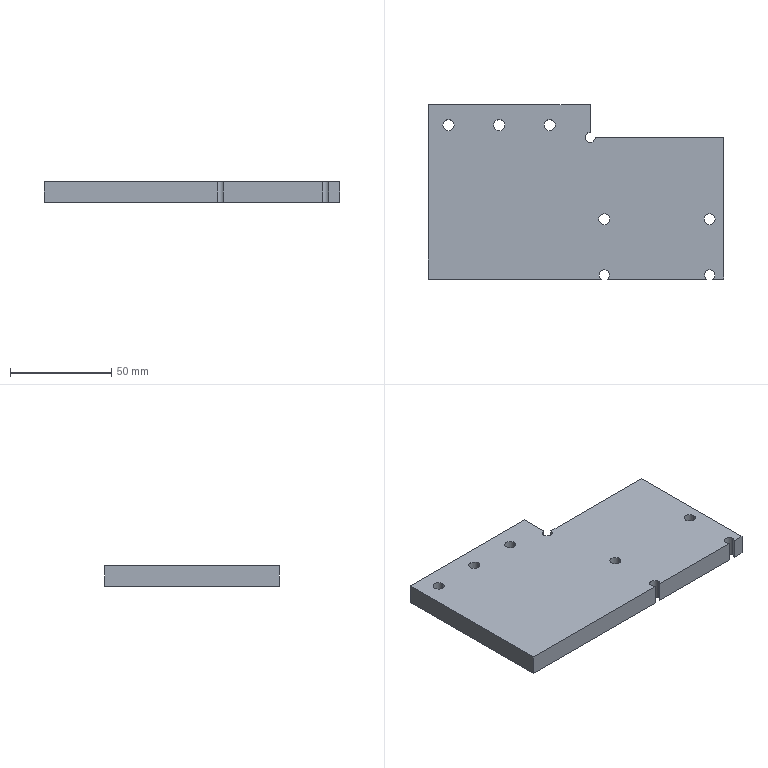Part | STEP file | 10-22Z轴连接块B | 1 solid | 43 faces | box 146 x 86 x 10 mm | volume 111813 mm3 | cylinder 28 | plane 15 | commonest cylinder face diameters 5.5 x10 10 x10 5 x8
STEP:
#1=CARTESIAN_POINT('',(16.5,-41.,10.));
#2=VERTEX_POINT('',#1);
#3=CARTESIAN_POINT('',(15.5,-43.,10.));
#4=VERTEX_POINT('',#3);
#5=CARTESIAN_POINT('',(14.,-41.,10.));
#6=DIRECTION('',(0.,0.,-1.));
#7=DIRECTION('',(-1.,0.,0.));
#8=AXIS2_PLACEMENT_3D('',#5,#6,#7);
#9=CIRCLE('',#8,2.5);
#10=EDGE_CURVE('',#2,#4,#9,.T.);
#11=ORIENTED_EDGE('',*,*,#10,.F.);
#12=CARTESIAN_POINT('',(16.5,-41.,0.));
#13=VERTEX_POINT('',#12);
#14=CARTESIAN_POINT('',(16.5,-41.,10.));
#15=DIRECTION('',(0.,0.,-1.));
#16=VECTOR('',#15,1000.);
#17=LINE('',#14,#16);
#18=EDGE_CURVE('',#2,#13,#17,.T.);
#19=ORIENTED_EDGE('',*,*,#18,.T.);
#20=CARTESIAN_POINT('',(15.5,-43.,0.));
#21=VERTEX_POINT('',#20);
#22=CARTESIAN_POINT('',(14.,-41.,0.));
#23=DIRECTION('',(0.,0.,1.));
#24=DIRECTION('',(1.,0.,0.));
#25=AXIS2_PLACEMENT_3D('',#22,#23,#24);
#26=CIRCLE('',#25,2.5);
#27=EDGE_CURVE('',#21,#13,#26,.T.);
#28=ORIENTED_EDGE('',*,*,#27,.F.);
#29=CARTESIAN_POINT('',(15.5,-43.,10.));
#30=DIRECTION('',(0.,0.,-1.));
#31=VECTOR('',#30,1000.);
#32=LINE('',#29,#31);
#33=EDGE_CURVE('',#4,#21,#32,.T.);
#34=ORIENTED_EDGE('',*,*,#33,.F.);
#35=EDGE_LOOP('',(#11,#19,#28,#34));
#36=FACE_OUTER_BOUND('',#35,.T.);
#37=CARTESIAN_POINT('',(14.,-41.,10.));
#38=DIRECTION('',(0.,0.,-1.));
#39=DIRECTION('',(-1.,0.,0.));
#40=AXIS2_PLACEMENT_3D('',#37,#38,#39);
#41=CYLINDRICAL_SURFACE('',#40,2.5);
#42=ADVANCED_FACE('',(#36),#41,.F.);
#43=ORIENTED_EDGE('',*,*,#18,.F.);
#44=CARTESIAN_POINT('',(11.5,-41.,10.));
#45=VERTEX_POINT('',#44);
#46=CARTESIAN_POINT('',(14.,-41.,10.));
#47=DIRECTION('',(0.,0.,-1.));
#48=DIRECTION('',(-1.,0.,0.));
#49=AXIS2_PLACEMENT_3D('',#46,#47,#48);
#50=CIRCLE('',#49,2.5);
#51=EDGE_CURVE('',#45,#2,#50,.T.);
#52=ORIENTED_EDGE('',*,*,#51,.F.);
#53=CARTESIAN_POINT('',(11.5,-41.,0.));
#54=VERTEX_POINT('',#53);
#55=CARTESIAN_POINT('',(11.5,-41.,10.));
#56=DIRECTION('',(0.,0.,-1.));
#57=VECTOR('',#56,1000.);
#58=LINE('',#55,#57);
#59=EDGE_CURVE('',#45,#54,#58,.T.);
#60=ORIENTED_EDGE('',*,*,#59,.T.);
#61=CARTESIAN_POINT('',(14.,-41.,0.));
#62=DIRECTION('',(0.,0.,1.));
#63=DIRECTION('',(1.,0.,0.));
#64=AXIS2_PLACEMENT_3D('',#61,#62,#63);
#65=CIRCLE('',#64,2.5);
#66=EDGE_CURVE('',#13,#54,#65,.T.);
#67=ORIENTED_EDGE('',*,*,#66,.F.);
#68=EDGE_LOOP('',(#43,#52,#60,#67));
#69=FACE_OUTER_BOUND('',#68,.T.);
#70=CARTESIAN_POINT('',(14.,-41.,10.));
#71=DIRECTION('',(0.,0.,-1.));
#72=DIRECTION('',(-1.,0.,0.));
#73=AXIS2_PLACEMENT_3D('',#70,#71,#72);
#74=CYLINDRICAL_SURFACE('',#73,2.5);
#75=ADVANCED_FACE('',(#69),#74,.F.);
#76=CARTESIAN_POINT('',(68.5,-41.,10.));
#77=VERTEX_POINT('',#76);
#78=CARTESIAN_POINT('',(67.5,-43.,10.));
#79=VERTEX_POINT('',#78);
#80=CARTESIAN_POINT('',(66.,-41.,10.));
#81=DIRECTION('',(0.,0.,-1.));
#82=DIRECTION('',(-1.,0.,0.));
#83=AXIS2_PLACEMENT_3D('',#80,#81,#82);
#84=CIRCLE('',#83,2.5);
#85=EDGE_CURVE('',#77,#79,#84,.T.);
#86=ORIENTED_EDGE('',*,*,#85,.F.);
#87=CARTESIAN_POINT('',(68.5,-41.,0.));
#88=VERTEX_POINT('',#87);
#89=CARTESIAN_POINT('',(68.5,-41.,10.));
#90=DIRECTION('',(0.,0.,-1.));
#91=VECTOR('',#90,1000.);
#92=LINE('',#89,#91);
#93=EDGE_CURVE('',#77,#88,#92,.T.);
#94=ORIENTED_EDGE('',*,*,#93,.T.);
#95=CARTESIAN_POINT('',(67.5,-43.,0.));
#96=VERTEX_POINT('',#95);
#97=CARTESIAN_POINT('',(66.,-41.,0.));
#98=DIRECTION('',(0.,0.,1.));
#99=DIRECTION('',(1.,0.,0.));
#100=AXIS2_PLACEMENT_3D('',#97,#98,#99);
#101=CIRCLE('',#100,2.5);
#102=EDGE_CURVE('',#96,#88,#101,.T.);
#103=ORIENTED_EDGE('',*,*,#102,.F.);
#104=CARTESIAN_POINT('',(67.5,-43.,10.));
#105=DIRECTION('',(0.,0.,-1.));
#106=VECTOR('',#105,1000.);
#107=LINE('',#104,#106);
#108=EDGE_CURVE('',#79,#96,#107,.T.);
#109=ORIENTED_EDGE('',*,*,#108,.F.);
#110=EDGE_LOOP('',(#86,#94,#103,#109));
#111=FACE_OUTER_BOUND('',#110,.T.);
#112=CARTESIAN_POINT('',(66.,-41.,10.));
#113=DIRECTION('',(0.,0.,-1.));
#114=DIRECTION('',(-1.,0.,0.));
#115=AXIS2_PLACEMENT_3D('',#112,#113,#114);
#116=CYLINDRICAL_SURFACE('',#115,2.5);
#117=ADVANCED_FACE('',(#111),#116,.F.);
#118=ORIENTED_EDGE('',*,*,#93,.F.);
#119=CARTESIAN_POINT('',(63.5,-41.,10.));
#120=VERTEX_POINT('',#119);
#121=CARTESIAN_POINT('',(66.,-41.,10.));
#122=DIRECTION('',(0.,0.,-1.));
#123=DIRECTION('',(-1.,0.,0.));
#124=AXIS2_PLACEMENT_3D('',#121,#122,#123);
#125=CIRCLE('',#124,2.5);
#126=EDGE_CURVE('',#120,#77,#125,.T.);
#127=ORIENTED_EDGE('',*,*,#126,.F.);
#128=CARTESIAN_POINT('',(63.5,-41.,0.));
#129=VERTEX_POINT('',#128);
#130=CARTESIAN_POINT('',(63.5,-41.,10.));
#131=DIRECTION('',(0.,0.,-1.));
#132=VECTOR('',#131,1000.);
#133=LINE('',#130,#132);
#134=EDGE_CURVE('',#120,#129,#133,.T.);
#135=ORIENTED_EDGE('',*,*,#134,.T.);
#136=CARTESIAN_POINT('',(66.,-41.,0.));
#137=DIRECTION('',(0.,0.,1.));
#138=DIRECTION('',(1.,0.,0.));
#139=AXIS2_PLACEMENT_3D('',#136,#137,#138);
#140=CIRCLE('',#139,2.5);
#141=EDGE_CURVE('',#88,#129,#140,.T.);
#142=ORIENTED_EDGE('',*,*,#141,.F.);
#143=EDGE_LOOP('',(#118,#127,#135,#142));
#144=FACE_OUTER_BOUND('',#143,.T.);
#145=CARTESIAN_POINT('',(66.,-41.,10.));
#146=DIRECTION('',(0.,0.,-1.));
#147=DIRECTION('',(-1.,0.,0.));
#148=AXIS2_PLACEMENT_3D('',#145,#146,#147);
#149=CYLINDRICAL_SURFACE('',#148,2.5);
#150=ADVANCED_FACE('',(#144),#149,.F.);
#151=CARTESIAN_POINT('',(71.,-13.5,5.4));
#152=VERTEX_POINT('',#151);
#153=CARTESIAN_POINT('',(61.,-13.5,5.4));
#154=VERTEX_POINT('',#153);
#155=CARTESIAN_POINT('',(66.,-13.5,5.4));
#156=DIRECTION('',(0.,0.,-1.));
#157=DIRECTION('',(-1.,0.,0.));
#158=AXIS2_PLACEMENT_3D('',#155,#156,#157);
#159=CIRCLE('',#158,5.);
#160=EDGE_CURVE('',#152,#154,#159,.T.);
#161=ORIENTED_EDGE('',*,*,#160,.F.);
#162=CARTESIAN_POINT('',(71.,-13.5,0.));
#163=VERTEX_POINT('',#162);
#164=CARTESIAN_POINT('',(71.,-13.5,0.));
#165=DIRECTION('',(0.,0.,-1.));
#166=VECTOR('',#165,1000.);
#167=LINE('',#164,#166);
#168=EDGE_CURVE('',#152,#163,#167,.T.);
#169=ORIENTED_EDGE('',*,*,#168,.T.);
#170=CARTESIAN_POINT('',(61.,-13.5,0.));
#171=VERTEX_POINT('',#170);
#172=CARTESIAN_POINT('',(66.,-13.5,0.));
#173=DIRECTION('',(0.,0.,-1.));
#174=DIRECTION('',(-1.,0.,0.));
#175=AXIS2_PLACEMENT_3D('',#172,#173,#174);
#176=CIRCLE('',#175,5.);
#177=EDGE_CURVE('',#163,#171,#176,.T.);
#178=ORIENTED_EDGE('',*,*,#177,.T.);
#179=CARTESIAN_POINT('',(61.,-13.5,0.));
#180=DIRECTION('',(0.,0.,-1.));
#181=VECTOR('',#180,1000.);
#182=LINE('',#179,#181);
#183=EDGE_CURVE('',#154,#171,#182,.T.);
#184=ORIENTED_EDGE('',*,*,#183,.F.);
#185=EDGE_LOOP('',(#161,#169,#178,#184));
#186=FACE_OUTER_BOUND('',#185,.T.);
#187=CARTESIAN_POINT('',(66.,-13.5,0.));
#188=DIRECTION('',(0.,0.,-1.));
#189=DIRECTION('',(-1.,0.,0.));
#190=AXIS2_PLACEMENT_3D('',#187,#188,#189);
#191=CYLINDRICAL_SURFACE('',#190,5.);
#192=ADVANCED_FACE('',(#186),#191,.F.);
#193=CARTESIAN_POINT('',(68.75,-13.5,10.));
#194=VERTEX_POINT('',#193);
#195=CARTESIAN_POINT('',(63.25,-13.5,10.));
#196=VERTEX_POINT('',#195);
#197=CARTESIAN_POINT('',(66.,-13.5,10.));
#198=DIRECTION('',(0.,0.,-1.));
#199=DIRECTION('',(-1.,0.,0.));
#200=AXIS2_PLACEMENT_3D('',#197,#198,#199);
#201=CIRCLE('',#200,2.75);
#202=EDGE_CURVE('',#194,#196,#201,.T.);
#203=ORIENTED_EDGE('',*,*,#202,.F.);
#204=CARTESIAN_POINT('',(68.75,-13.5,5.4));
#205=VERTEX_POINT('',#204);
#206=CARTESIAN_POINT('',(68.75,-13.5,0.));
#207=DIRECTION('',(0.,0.,-1.));
#208=VECTOR('',#207,1000.);
#209=LINE('',#206,#208);
#210=EDGE_CURVE('',#194,#205,#209,.T.);
#211=ORIENTED_EDGE('',*,*,#210,.T.);
#212=CARTESIAN_POINT('',(63.25,-13.5,5.4));
#213=VERTEX_POINT('',#212);
#214=CARTESIAN_POINT('',(66.,-13.5,5.4));
#215=DIRECTION('',(0.,0.,-1.));
#216=DIRECTION('',(-1.,0.,0.));
#217=AXIS2_PLACEMENT_3D('',#214,#215,#216);
#218=CIRCLE('',#217,2.75);
#219=EDGE_CURVE('',#205,#213,#218,.T.);
#220=ORIENTED_EDGE('',*,*,#219,.T.);
#221=CARTESIAN_POINT('',(63.25,-13.5,0.));
#222=DIRECTION('',(0.,0.,-1.));
#223=VECTOR('',#222,1000.);
#224=LINE('',#221,#223);
#225=EDGE_CURVE('',#196,#213,#224,.T.);
#226=ORIENTED_EDGE('',*,*,#225,.F.);
#227=EDGE_LOOP('',(#203,#211,#220,#226));
#228=FACE_OUTER_BOUND('',#227,.T.);
#229=CARTESIAN_POINT('',(66.,-13.5,0.));
#230=DIRECTION('',(0.,0.,-1.));
#231=DIRECTION('',(-1.,0.,0.));
#232=AXIS2_PLACEMENT_3D('',#229,#230,#231);
#233=CYLINDRICAL_SURFACE('',#232,2.75);
#234=ADVANCED_FACE('',(#228),#233,.F.);
#235=CARTESIAN_POINT('',(19.,-13.5,5.4));
#236=VERTEX_POINT('',#235);
#237=CARTESIAN_POINT('',(9.,-13.5,5.4));
#238=VERTEX_POINT('',#237);
#239=CARTESIAN_POINT('',(14.,-13.5,5.4));
#240=DIRECTION('',(0.,0.,-1.));
#241=DIRECTION('',(-1.,0.,0.));
#242=AXIS2_PLACEMENT_3D('',#239,#240,#241);
#243=CIRCLE('',#242,5.);
#244=EDGE_CURVE('',#236,#238,#243,.T.);
#245=ORIENTED_EDGE('',*,*,#244,.F.);
#246=CARTESIAN_POINT('',(19.,-13.5,0.));
#247=VERTEX_POINT('',#246);
#248=CARTESIAN_POINT('',(19.,-13.5,0.));
#249=DIRECTION('',(0.,0.,-1.));
#250=VECTOR('',#249,1000.);
#251=LINE('',#248,#250);
#252=EDGE_CURVE('',#236,#247,#251,.T.);
#253=ORIENTED_EDGE('',*,*,#252,.T.);
#254=CARTESIAN_POINT('',(9.,-13.5,0.));
#255=VERTEX_POINT('',#254);
#256=CARTESIAN_POINT('',(14.,-13.5,0.));
#257=DIRECTION('',(0.,0.,-1.));
#258=DIRECTION('',(-1.,0.,0.));
#259=AXIS2_PLACEMENT_3D('',#256,#257,#258);
#260=CIRCLE('',#259,5.);
#261=EDGE_CURVE('',#247,#255,#260,.T.);
#262=ORIENTED_EDGE('',*,*,#261,.T.);
#263=CARTESIAN_POINT('',(9.,-13.5,0.));
#264=DIRECTION('',(0.,0.,-1.));
#265=VECTOR('',#264,1000.);
#266=LINE('',#263,#265);
#267=EDGE_CURVE('',#238,#255,#266,.T.);
#268=ORIENTED_EDGE('',*,*,#267,.F.);
#269=EDGE_LOOP('',(#245,#253,#262,#268));
#270=FACE_OUTER_BOUND('',#269,.T.);
#271=CARTESIAN_POINT('',(14.,-13.5,0.));
#272=DIRECTION('',(0.,0.,-1.));
#273=DIRECTION('',(-1.,0.,0.));
#274=AXIS2_PLACEMENT_3D('',#271,#272,#273);
#275=CYLINDRICAL_SURFACE('',#274,5.);
#276=ADVANCED_FACE('',(#270),#275,.F.);
#277=CARTESIAN_POINT('',(16.75,-13.5,10.));
#278=VERTEX_POINT('',#277);
#279=CARTESIAN_POINT('',(11.25,-13.5,10.));
#280=VERTEX_POINT('',#279);
#281=CARTESIAN_POINT('',(14.,-13.5,10.));
#282=DIRECTION('',(0.,0.,-1.));
#283=DIRECTION('',(-1.,0.,0.));
#284=AXIS2_PLACEMENT_3D('',#281,#282,#283);
#285=CIRCLE('',#284,2.75);
#286=EDGE_CURVE('',#278,#280,#285,.T.);
#287=ORIENTED_EDGE('',*,*,#286,.F.);
#288=CARTESIAN_POINT('',(16.75,-13.5,5.4));
#289=VERTEX_POINT('',#288);
#290=CARTESIAN_POINT('',(16.75,-13.5,0.));
#291=DIRECTION('',(0.,0.,-1.));
#292=VECTOR('',#291,1000.);
#293=LINE('',#290,#292);
#294=EDGE_CURVE('',#278,#289,#293,.T.);
#295=ORIENTED_EDGE('',*,*,#294,.T.);
#296=CARTESIAN_POINT('',(11.25,-13.5,5.4));
#297=VERTEX_POINT('',#296);
#298=CARTESIAN_POINT('',(14.,-13.5,5.4));
#299=DIRECTION('',(0.,0.,-1.));
#300=DIRECTION('',(-1.,0.,0.));
#301=AXIS2_PLACEMENT_3D('',#298,#299,#300);
#302=CIRCLE('',#301,2.75);
#303=EDGE_CURVE('',#289,#297,#302,.T.);
#304=ORIENTED_EDGE('',*,*,#303,.T.);
#305=CARTESIAN_POINT('',(11.25,-13.5,0.));
#306=DIRECTION('',(0.,0.,-1.));
#307=VECTOR('',#306,1000.);
#308=LINE('',#305,#307);
#309=EDGE_CURVE('',#280,#297,#308,.T.);
#310=ORIENTED_EDGE('',*,*,#309,.F.);
#311=EDGE_LOOP('',(#287,#295,#304,#310));
#312=FACE_OUTER_BOUND('',#311,.T.);
#313=CARTESIAN_POINT('',(14.,-13.5,0.));
#314=DIRECTION('',(0.,0.,-1.));
#315=DIRECTION('',(-1.,0.,0.));
#316=AXIS2_PLACEMENT_3D('',#313,#314,#315);
#317=CYLINDRICAL_SURFACE('',#316,2.75);
#318=ADVANCED_FACE('',(#312),#317,.F.);
#319=CARTESIAN_POINT('',(-58.,33.,5.4));
#320=VERTEX_POINT('',#319);
#321=CARTESIAN_POINT('',(-68.,33.,5.4));
#322=VERTEX_POINT('',#321);
#323=CARTESIAN_POINT('',(-63.,33.,5.4));
#324=DIRECTION('',(0.,0.,-1.));
#325=DIRECTION('',(-1.,0.,0.));
#326=AXIS2_PLACEMENT_3D('',#323,#324,#325);
#327=CIRCLE('',#326,5.);
#328=EDGE_CURVE('',#320,#322,#327,.T.);
#329=ORIENTED_EDGE('',*,*,#328,.F.);
#330=CARTESIAN_POINT('',(-58.,33.,0.));
#331=VERTEX_POINT('',#330);
#332=CARTESIAN_POINT('',(-58.,33.,0.));
#333=DIRECTION('',(0.,0.,-1.));
#334=VECTOR('',#333,1000.);
#335=LINE('',#332,#334);
#336=EDGE_CURVE('',#320,#331,#335,.T.);
#337=ORIENTED_EDGE('',*,*,#336,.T.);
#338=CARTESIAN_POINT('',(-68.,33.,0.));
#339=VERTEX_POINT('',#338);
#340=CARTESIAN_POINT('',(-63.,33.,0.));
#341=DIRECTION('',(0.,0.,-1.));
#342=DIRECTION('',(-1.,0.,0.));
#343=AXIS2_PLACEMENT_3D('',#340,#341,#342);
#344=CIRCLE('',#343,5.);
#345=EDGE_CURVE('',#331,#339,#344,.T.);
#346=ORIENTED_EDGE('',*,*,#345,.T.);
#347=CARTESIAN_POINT('',(-68.,33.,0.));
#348=DIRECTION('',(0.,0.,-1.));
#349=VECTOR('',#348,1000.);
#350=LINE('',#347,#349);
#351=EDGE_CURVE('',#322,#339,#350,.T.);
#352=ORIENTED_EDGE('',*,*,#351,.F.);
#353=EDGE_LOOP('',(#329,#337,#346,#352));
#354=FACE_OUTER_BOUND('',#353,.T.);
#355=CARTESIAN_POINT('',(-63.,33.,0.));
#356=DIRECTION('',(0.,0.,-1.));
#357=DIRECTION('',(-1.,0.,0.));
#358=AXIS2_PLACEMENT_3D('',#355,#356,#357);
#359=CYLINDRICAL_SURFACE('',#358,5.);
#360=ADVANCED_FACE('',(#354),#359,.F.);
#361=CARTESIAN_POINT('',(-60.25,33.,10.));
#362=VERTEX_POINT('',#361);
#363=CARTESIAN_POINT('',(-65.75,33.,10.));
#364=VERTEX_POINT('',#363);
#365=CARTESIAN_POINT('',(-63.,33.,10.));
#366=DIRECTION('',(0.,0.,-1.));
#367=DIRECTION('',(-1.,0.,0.));
#368=AXIS2_PLACEMENT_3D('',#365,#366,#367);
#369=CIRCLE('',#368,2.75);
#370=EDGE_CURVE('',#362,#364,#369,.T.);
#371=ORIENTED_EDGE('',*,*,#370,.F.);
#372=CARTESIAN_POINT('',(-60.25,33.,5.4));
#373=VERTEX_POINT('',#372);
#374=CARTESIAN_POINT('',(-60.25,33.,0.));
#375=DIRECTION('',(0.,0.,-1.));
#376=VECTOR('',#375,1000.);
#377=LINE('',#374,#376);
#378=EDGE_CURVE('',#362,#373,#377,.T.);
#379=ORIENTED_EDGE('',*,*,#378,.T.);
#380=CARTESIAN_POINT('',(-65.75,33.,5.4));
#381=VERTEX_POINT('',#380);
#382=CARTESIAN_POINT('',(-63.,33.,5.4));
#383=DIRECTION('',(0.,0.,-1.));
#384=DIRECTION('',(-1.,0.,0.));
#385=AXIS2_PLACEMENT_3D('',#382,#383,#384);
#386=CIRCLE('',#385,2.75);
#387=EDGE_CURVE('',#373,#381,#386,.T.);
#388=ORIENTED_EDGE('',*,*,#387,.T.);
#389=CARTESIAN_POINT('',(-65.75,33.,0.));
#390=DIRECTION('',(0.,0.,-1.));
#391=VECTOR('',#390,1000.);
#392=LINE('',#389,#391);
#393=EDGE_CURVE('',#364,#381,#392,.T.);
#394=ORIENTED_EDGE('',*,*,#393,.F.);
#395=EDGE_LOOP('',(#371,#379,#388,#394));
#396=FACE_OUTER_BOUND('',#395,.T.);
#397=CARTESIAN_POINT('',(-63.,33.,0.));
#398=DIRECTION('',(0.,0.,-1.));
#399=DIRECTION('',(-1.,0.,0.));
#400=AXIS2_PLACEMENT_3D('',#397,#398,#399);
#401=CYLINDRICAL_SURFACE('',#400,2.75);
#402=ADVANCED_FACE('',(#396),#401,.F.);
#403=CARTESIAN_POINT('',(-33.,33.,5.4));
#404=VERTEX_POINT('',#403);
#405=CARTESIAN_POINT('',(-43.,33.,5.4));
#406=VERTEX_POINT('',#405);
#407=CARTESIAN_POINT('',(-38.,33.,5.4));
#408=DIRECTION('',(0.,0.,-1.));
#409=DIRECTION('',(-1.,0.,0.));
#410=AXIS2_PLACEMENT_3D('',#407,#408,#409);
#411=CIRCLE('',#410,5.);
#412=EDGE_CURVE('',#404,#406,#411,.T.);
#413=ORIENTED_EDGE('',*,*,#412,.F.);
#414=CARTESIAN_POINT('',(-33.,33.,0.));
#415=VERTEX_POINT('',#414);
#416=CARTESIAN_POINT('',(-33.,33.,0.));
#417=DIRECTION('',(0.,0.,-1.));
#418=VECTOR('',#417,1000.);
#419=LINE('',#416,#418);
#420=EDGE_CURVE('',#404,#415,#419,.T.);
#421=ORIENTED_EDGE('',*,*,#420,.T.);
#422=CARTESIAN_POINT('',(-43.,33.,0.));
#423=VERTEX_POINT('',#422);
#424=CARTESIAN_POINT('',(-38.,33.,0.));
#425=DIRECTION('',(0.,0.,-1.));
#426=DIRECTION('',(-1.,0.,0.));
#427=AXIS2_PLACEMENT_3D('',#424,#425,#426);
#428=CIRCLE('',#427,5.);
#429=EDGE_CURVE('',#415,#423,#428,.T.);
#430=ORIENTED_EDGE('',*,*,#429,.T.);
#431=CARTESIAN_POINT('',(-43.,33.,0.));
#432=DIRECTION('',(0.,0.,-1.));
#433=VECTOR('',#432,1000.);
#434=LINE('',#431,#433);
#435=EDGE_CURVE('',#406,#423,#434,.T.);
#436=ORIENTED_EDGE('',*,*,#435,.F.);
#437=EDGE_LOOP('',(#413,#421,#430,#436));
#438=FACE_OUTER_BOUND('',#437,.T.);
#439=CARTESIAN_POINT('',(-38.,33.,0.));
#440=DIRECTION('',(0.,0.,-1.));
#441=DIRECTION('',(-1.,0.,0.));
#442=AXIS2_PLACEMENT_3D('',#439,#440,#441);
#443=CYLINDRICAL_SURFACE('',#442,5.);
#444=ADVANCED_FACE('',(#438),#443,.F.);
#445=CARTESIAN_POINT('',(-35.25,33.,10.));
#446=VERTEX_POINT('',#445);
#447=CARTESIAN_POINT('',(-40.75,33.,10.));
#448=VERTEX_POINT('',#447);
#449=CARTESIAN_POINT('',(-38.,33.,10.));
#450=DIRECTION('',(0.,0.,-1.));
#451=DIRECTION('',(-1.,0.,0.));
#452=AXIS2_PLACEMENT_3D('',#449,#450,#451);
#453=CIRCLE('',#452,2.75);
#454=EDGE_CURVE('',#446,#448,#453,.T.);
#455=ORIENTED_EDGE('',*,*,#454,.F.);
#456=CARTESIAN_POINT('',(-35.25,33.,5.4));
#457=VERTEX_POINT('',#456);
#458=CARTESIAN_POINT('',(-35.25,33.,0.));
#459=DIRECTION('',(0.,0.,-1.));
#460=VECTOR('',#459,1000.);
#461=LINE('',#458,#460);
#462=EDGE_CURVE('',#446,#457,#461,.T.);
#463=ORIENTED_EDGE('',*,*,#462,.T.);
#464=CARTESIAN_POINT('',(-40.75,33.,5.4));
#465=VERTEX_POINT('',#464);
#466=CARTESIAN_POINT('',(-38.,33.,5.4));
#467=DIRECTION('',(0.,0.,-1.));
#468=DIRECTION('',(-1.,0.,0.));
#469=AXIS2_PLACEMENT_3D('',#466,#467,#468);
#470=CIRCLE('',#469,2.75);
#471=EDGE_CURVE('',#457,#465,#470,.T.);
#472=ORIENTED_EDGE('',*,*,#471,.T.);
#473=CARTESIAN_POINT('',(-40.75,33.,0.));
#474=DIRECTION('',(0.,0.,-1.));
#475=VECTOR('',#474,1000.);
#476=LINE('',#473,#475);
#477=EDGE_CURVE('',#448,#465,#476,.T.);
#478=ORIENTED_EDGE('',*,*,#477,.F.);
#479=EDGE_LOOP('',(#455,#463,#472,#478));
#480=FACE_OUTER_BOUND('',#479,.T.);
#481=CARTESIAN_POINT('',(-38.,33.,0.));
#482=DIRECTION('',(0.,0.,-1.));
#483=DIRECTION('',(-1.,0.,0.));
#484=AXIS2_PLACEMENT_3D('',#481,#482,#483);
#485=CYLINDRICAL_SURFACE('',#484,2.75);
#486=ADVANCED_FACE('',(#480),#485,.F.);
#487=CARTESIAN_POINT('',(-8.,33.,5.4));
#488=VERTEX_POINT('',#487);
#489=CARTESIAN_POINT('',(-18.,33.,5.4));
#490=VERTEX_POINT('',#489);
#491=CARTESIAN_POINT('',(-13.,33.,5.4));
#492=DIRECTION('',(0.,0.,-1.));
#493=DIRECTION('',(-1.,0.,0.));
#494=AXIS2_PLACEMENT_3D('',#491,#492,#493);
#495=CIRCLE('',#494,5.);
#496=EDGE_CURVE('',#488,#490,#495,.T.);
#497=ORIENTED_EDGE('',*,*,#496,.F.);
#498=CARTESIAN_POINT('',(-8.,33.,0.));
#499=VERTEX_POINT('',#498);
#500=CARTESIAN_POINT('',(-8.,33.,0.));
#501=DIRECTION('',(0.,0.,-1.));
#502=VECTOR('',#501,1000.);
#503=LINE('',#500,#502);
#504=EDGE_CURVE('',#488,#499,#503,.T.);
#505=ORIENTED_EDGE('',*,*,#504,.T.);
#506=CARTESIAN_POINT('',(-18.,33.,0.));
#507=VERTEX_POINT('',#506);
#508=CARTESIAN_POINT('',(-13.,33.,0.));
#509=DIRECTION('',(0.,0.,-1.));
#510=DIRECTION('',(-1.,0.,0.));
#511=AXIS2_PLACEMENT_3D('',#508,#509,#510);
#512=CIRCLE('',#511,5.);
#513=EDGE_CURVE('',#499,#507,#512,.T.);
#514=ORIENTED_EDGE('',*,*,#513,.T.);
#515=CARTESIAN_POINT('',(-18.,33.,0.));
#516=DIRECTION('',(0.,0.,-1.));
#517=VECTOR('',#516,1000.);
#518=LINE('',#515,#517);
#519=EDGE_CURVE('',#490,#507,#518,.T.);
#520=ORIENTED_EDGE('',*,*,#519,.F.);
#521=EDGE_LOOP('',(#497,#505,#514,#520));
#522=FACE_OUTER_BOUND('',#521,.T.);
#523=CARTESIAN_POINT('',(-13.,33.,0.));
#524=DIRECTION('',(0.,0.,-1.));
#525=DIRECTION('',(-1.,0.,0.));
#526=AXIS2_PLACEMENT_3D('',#523,#524,#525);
#527=CYLINDRICAL_SURFACE('',#526,5.);
#528=ADVANCED_FACE('',(#522),#527,.F.);
#529=CARTESIAN_POINT('',(-10.25,33.,10.));
#530=VERTEX_POINT('',#529);
#531=CARTESIAN_POINT('',(-15.75,33.,10.));
#532=VERTEX_POINT('',#531);
#533=CARTESIAN_POINT('',(-13.,33.,10.));
#534=DIRECTION('',(0.,0.,-1.));
#535=DIRECTION('',(-1.,0.,0.));
#536=AXIS2_PLACEMENT_3D('',#533,#534,#535);
#537=CIRCLE('',#536,2.75);
#538=EDGE_CURVE('',#530,#532,#537,.T.);
#539=ORIENTED_EDGE('',*,*,#538,.F.);
#540=CARTESIAN_POINT('',(-10.25,33.,5.4));
#541=VERTEX_POINT('',#540);
#542=CARTESIAN_POINT('',(-10.25,33.,0.));
#543=DIRECTION('',(0.,0.,-1.));
#544=VECTOR('',#543,1000.);
#545=LINE('',#542,#544);
#546=EDGE_CURVE('',#530,#541,#545,.T.);
#547=ORIENTED_EDGE('',*,*,#546,.T.);
#548=CARTESIAN_POINT('',(-15.75,33.,5.4));
#549=VERTEX_POINT('',#548);
#550=CARTESIAN_POINT('',(-13.,33.,5.4));
#551=DIRECTION('',(0.,0.,-1.));
#552=DIRECTION('',(-1.,0.,0.));
#553=AXIS2_PLACEMENT_3D('',#550,#551,#552);
#554=CIRCLE('',#553,2.75);
#555=EDGE_CURVE('',#541,#549,#554,.T.);
#556=ORIENTED_EDGE('',*,*,#555,.T.);
#557=CARTESIAN_POINT('',(-15.75,33.,0.));
#558=DIRECTION('',(0.,0.,-1.));
#559=VECTOR('',#558,1000.);
#560=LINE('',#557,#559);
#561=EDGE_CURVE('',#532,#549,#560,.T.);
#562=ORIENTED_EDGE('',*,*,#561,.F.);
#563=EDGE_LOOP('',(#539,#547,#556,#562));
#564=FACE_OUTER_BOUND('',#563,.T.);
#565=CARTESIAN_POINT('',(-13.,33.,0.));
#566=DIRECTION('',(0.,0.,-1.));
#567=DIRECTION('',(-1.,0.,0.));
#568=AXIS2_PLACEMENT_3D('',#565,#566,#567);
#569=CYLINDRICAL_SURFACE('',#568,2.75);
#570=ADVANCED_FACE('',(#564),#569,.F.);
#571=CARTESIAN_POINT('',(4.5,27.,10.));
#572=VERTEX_POINT('',#571);
#573=CARTESIAN_POINT('',(7.,29.5,10.));
#574=VERTEX_POINT('',#573);
#575=CARTESIAN_POINT('',(7.,27.,10.));
#576=DIRECTION('',(0.,0.,-1.));
#577=DIRECTION('',(-1.,0.,0.));
#578=AXIS2_PLACEMENT_3D('',#575,#576,#577);
#579=CIRCLE('',#578,2.5);
#580=EDGE_CURVE('',#572,#574,#579,.T.);
#581=ORIENTED_EDGE('',*,*,#580,.F.);
#582=CARTESIAN_POINT('',(4.5,27.,0.));
#583=VERTEX_POINT('',#582);
#584=CARTESIAN_POINT('',(4.5,27.,10.));
#585=DIRECTION('',(0.,0.,-1.));
#586=VECTOR('',#585,1000.);
#587=LINE('',#584,#586);
#588=EDGE_CURVE('',#572,#583,#587,.T.);
#589=ORIENTED_EDGE('',*,*,#588,.T.);
#590=CARTESIAN_POINT('',(7.,29.5,0.));
#591=VERTEX_POINT('',#590);
#592=CARTESIAN_POINT('',(7.,27.,0.));
#593=DIRECTION('',(0.,0.,-1.));
#594=DIRECTION('',(-1.,0.,0.));
#595=AXIS2_PLACEMENT_3D('',#592,#593,#594);
#596=CIRCLE('',#595,2.5);
#597=EDGE_CURVE('',#583,#591,#596,.T.);
#598=ORIENTED_EDGE('',*,*,#597,.T.);
#599=CARTESIAN_POINT('',(7.,29.5,10.));
#600=DIRECTION('',(0.,0.,-1.));
#601=VECTOR('',#600,1000.);
#602=LINE('',#599,#601);
#603=EDGE_CURVE('',#574,#591,#602,.T.);
#604=ORIENTED_EDGE('',*,*,#603,.F.);
#605=EDGE_LOOP('',(#581,#589,#598,#604));
#606=FACE_OUTER_BOUND('',#605,.T.);
#607=CARTESIAN_POINT('',(7.,27.,10.));
#608=DIRECTION('',(0.,0.,-1.));
#609=DIRECTION('',(-1.,0.,0.));
#610=AXIS2_PLACEMENT_3D('',#607,#608,#609);
#611=CYLINDRICAL_SURFACE('',#610,2.5);
#612=ADVANCED_FACE('',(#606),#611,.F.);
#613=CARTESIAN_POINT('',(64.5,-43.,10.));
#614=VERTEX_POINT('',#613);
#615=CARTESIAN_POINT('',(-73.,-43.,10.));
#616=DIRECTION('',(1.,0.,0.));
#617=VECTOR('',#616,1000.);
#618=LINE('',#615,#617);
#619=EDGE_CURVE('',#4,#614,#618,.T.);
#620=ORIENTED_EDGE('',*,*,#619,.F.);
#621=ORIENTED_EDGE('',*,*,#33,.T.);
#622=CARTESIAN_POINT('',(64.5,-43.,0.));
#623=VERTEX_POINT('',#622);
#624=CARTESIAN_POINT('',(-73.,-43.,0.));
#625=DIRECTION('',(1.,0.,0.));
#626=VECTOR('',#625,1000.);
#627=LINE('',#624,#626);
#628=EDGE_CURVE('',#21,#623,#627,.T.);
#629=ORIENTED_EDGE('',*,*,#628,.T.);
#630=CARTESIAN_POINT('',(64.5,-43.,10.));
#631=DIRECTION('',(0.,0.,1.));
#632=VECTOR('',#631,1000.);
#633=LINE('',#630,#632);
#634=EDGE_CURVE('',#623,#614,#633,.T.);
#635=ORIENTED_EDGE('',*,*,#634,.T.);
#636=EDGE_LOOP('',(#620,#621,#629,#635));
#637=FACE_OUTER_BOUND('',#636,.T.);
#638=CARTESIAN_POINT('',(-73.,-43.,10.));
#639=DIRECTION('',(0.,1.,0.));
#640=DIRECTION('',(0.,0.,1.));
#641=AXIS2_PLACEMENT_3D('',#638,#639,#640);
#642=PLANE('',#641);
#643=ADVANCED_FACE('',(#637),#642,.F.);
#644=CARTESIAN_POINT('',(73.,-43.,10.));
#645=VERTEX_POINT('',#644);
#646=CARTESIAN_POINT('',(-73.,-43.,10.));
#647=DIRECTION('',(1.,0.,0.));
#648=VECTOR('',#647,1000.);
#649=LINE('',#646,#648);
#650=EDGE_CURVE('',#79,#645,#649,.T.);
#651=ORIENTED_EDGE('',*,*,#650,.F.);
#652=ORIENTED_EDGE('',*,*,#108,.T.);
#653=CARTESIAN_POINT('',(73.,-43.,0.));
#654=VERTEX_POINT('',#653);
#655=CARTESIAN_POINT('',(-73.,-43.,0.));
#656=DIRECTION('',(1.,0.,0.));
#657=VECTOR('',#656,1000.);
#658=LINE('',#655,#657);
#659=EDGE_CURVE('',#96,#654,#658,.T.);
#660=ORIENTED_EDGE('',*,*,#659,.T.);
#661=CARTESIAN_POINT('',(73.,-43.,10.));
#662=DIRECTION('',(0.,0.,-1.));
#663=VECTOR('',#662,1000.);
#664=LINE('',#661,#663);
#665=EDGE_CURVE('',#645,#654,#664,.T.);
#666=ORIENTED_EDGE('',*,*,#665,.F.);
#667=EDGE_LOOP('',(#651,#652,#660,#666));
#668=FACE_OUTER_BOUND('',#667,.T.);
#669=CARTESIAN_POINT('',(-73.,-43.,10.));
#670=DIRECTION('',(0.,1.,0.));
#671=DIRECTION('',(0.,0.,1.));
#672=AXIS2_PLACEMENT_3D('',#669,#670,#671);
#673=PLANE('',#672);
#674=ADVANCED_FACE('',(#668),#673,.F.);
#675=CARTESIAN_POINT('',(73.,27.,0.));
#676=VERTEX_POINT('',#675);
#677=CARTESIAN_POINT('',(73.,43.,0.));
#678=DIRECTION('',(0.,1.,0.));
#679=VECTOR('',#678,1000.);
#680=LINE('',#677,#679);
#681=EDGE_CURVE('',#654,#676,#680,.T.);
#682=ORIENTED_EDGE('',*,*,#681,.T.);
#683=CARTESIAN_POINT('',(73.,27.,10.));
#684=VERTEX_POINT('',#683);
#685=CARTESIAN_POINT('',(73.,27.,10.));
#686=DIRECTION('',(0.,0.,-1.));
#687=VECTOR('',#686,1000.);
#688=LINE('',#685,#687);
#689=EDGE_CURVE('',#684,#676,#688,.T.);
#690=ORIENTED_EDGE('',*,*,#689,.F.);
#691=CARTESIAN_POINT('',(73.,43.,10.));
#692=DIRECTION('',(0.,1.,0.));
#693=VECTOR('',#692,1000.);
#694=LINE('',#691,#693);
#695=EDGE_CURVE('',#645,#684,#694,.T.);
#696=ORIENTED_EDGE('',*,*,#695,.F.);
#697=ORIENTED_EDGE('',*,*,#665,.T.);
#698=EDGE_LOOP('',(#682,#690,#696,#697));
#699=FACE_OUTER_BOUND('',#698,.T.);
#700=CARTESIAN_POINT('',(73.,43.,10.));
#701=DIRECTION('',(-1.,0.,0.));
#702=DIRECTION('',(0.,-1.,0.));
#703=AXIS2_PLACEMENT_3D('',#700,#701,#702);
#704=PLANE('',#703);
#705=ADVANCED_FACE('',(#699),#704,.F.);
#706=CARTESIAN_POINT('',(7.,43.,10.));
#707=VERTEX_POINT('',#706);
#708=CARTESIAN_POINT('',(-73.,43.,10.));
#709=VERTEX_POINT('',#708);
#710=CARTESIAN_POINT('',(-73.,43.,10.));
#711=DIRECTION('',(-1.,0.,0.));
#712=VECTOR('',#711,1000.);
#713=LINE('',#710,#712);
#714=EDGE_CURVE('',#707,#709,#713,.T.);
#715=ORIENTED_EDGE('',*,*,#714,.F.);
#716=CARTESIAN_POINT('',(7.,43.,0.));
#717=VERTEX_POINT('',#716);
#718=CARTESIAN_POINT('',(7.,43.,10.));
#719=DIRECTION('',(0.,0.,-1.));
#720=VECTOR('',#719,1000.);
#721=LINE('',#718,#720);
#722=EDGE_CURVE('',#707,#717,#721,.T.);
#723=ORIENTED_EDGE('',*,*,#722,.T.);
#724=CARTESIAN_POINT('',(-73.,43.,0.));
#725=VERTEX_POINT('',#724);
#726=CARTESIAN_POINT('',(-73.,43.,0.));
#727=DIRECTION('',(-1.,0.,0.));
#728=VECTOR('',#727,1000.);
#729=LINE('',#726,#728);
#730=EDGE_CURVE('',#717,#725,#729,.T.);
#731=ORIENTED_EDGE('',*,*,#730,.T.);
#732=CARTESIAN_POINT('',(-73.,43.,10.));
#733=DIRECTION('',(0.,0.,-1.));
#734=VECTOR('',#733,1000.);
#735=LINE('',#732,#734);
#736=EDGE_CURVE('',#709,#725,#735,.T.);
#737=ORIENTED_EDGE('',*,*,#736,.F.);
#738=EDGE_LOOP('',(#715,#723,#731,#737));
#739=FACE_OUTER_BOUND('',#738,.T.);
#740=CARTESIAN_POINT('',(-73.,43.,10.));
#741=DIRECTION('',(0.,-1.,0.));
#742=DIRECTION('',(0.,0.,-1.));
#743=AXIS2_PLACEMENT_3D('',#740,#741,#742);
#744=PLANE('',#743);
#745=ADVANCED_FACE('',(#739),#744,.F.);
#746=CARTESIAN_POINT('',(-73.,-43.,0.));
#747=VERTEX_POINT('',#746);
#748=CARTESIAN_POINT('',(-73.,43.,0.));
#749=DIRECTION('',(0.,-1.,0.));
#750=VECTOR('',#749,1000.);
#751=LINE('',#748,#750);
#752=EDGE_CURVE('',#725,#747,#751,.T.);
#753=ORIENTED_EDGE('',*,*,#752,.T.);
#754=CARTESIAN_POINT('',(-73.,-43.,10.));
#755=VERTEX_POINT('',#754);
#756=CARTESIAN_POINT('',(-73.,-43.,10.));
#757=DIRECTION('',(0.,0.,-1.));
#758=VECTOR('',#757,1000.);
#759=LINE('',#756,#758);
#760=EDGE_CURVE('',#755,#747,#759,.T.);
#761=ORIENTED_EDGE('',*,*,#760,.F.);
#762=CARTESIAN_POINT('',(-73.,43.,10.));
#763=DIRECTION('',(0.,-1.,0.));
#764=VECTOR('',#763,1000.);
#765=LINE('',#762,#764);
#766=EDGE_CURVE('',#709,#755,#765,.T.);
#767=ORIENTED_EDGE('',*,*,#766,.F.);
#768=ORIENTED_EDGE('',*,*,#736,.T.);
#769=EDGE_LOOP('',(#753,#761,#767,#768));
#770=FACE_OUTER_BOUND('',#769,.T.);
#771=CARTESIAN_POINT('',(-73.,43.,10.));
#772=DIRECTION('',(1.,0.,0.));
#773=DIRECTION('',(0.,1.,0.));
#774=AXIS2_PLACEMENT_3D('',#771,#772,#773);
#775=PLANE('',#774);
#776=ADVANCED_FACE('',(#770),#775,.F.);
#777=CARTESIAN_POINT('',(12.5,-43.,0.));
#778=VERTEX_POINT('',#777);
#779=CARTESIAN_POINT('',(-73.,-43.,0.));
#780=DIRECTION('',(1.,0.,0.));
#781=VECTOR('',#780,1000.);
#782=LINE('',#779,#781);
#783=EDGE_CURVE('',#747,#778,#782,.T.);
#784=ORIENTED_EDGE('',*,*,#783,.T.);
#785=CARTESIAN_POINT('',(12.5,-43.,10.));
#786=VERTEX_POINT('',#785);
#787=CARTESIAN_POINT('',(12.5,-43.,10.));
#788=DIRECTION('',(0.,0.,1.));
#789=VECTOR('',#788,1000.);
#790=LINE('',#787,#789);
#791=EDGE_CURVE('',#778,#786,#790,.T.);
#792=ORIENTED_EDGE('',*,*,#791,.T.);
#793=CARTESIAN_POINT('',(-73.,-43.,10.));
#794=DIRECTION('',(1.,0.,0.));
#795=VECTOR('',#794,1000.);
#796=LINE('',#793,#795);
#797=EDGE_CURVE('',#755,#786,#796,.T.);
#798=ORIENTED_EDGE('',*,*,#797,.F.);
#799=ORIENTED_EDGE('',*,*,#760,.T.);
#800=EDGE_LOOP('',(#784,#792,#798,#799));
#801=FACE_OUTER_BOUND('',#800,.T.);
#802=CARTESIAN_POINT('',(-73.,-43.,10.));
#803=DIRECTION('',(0.,1.,0.));
#804=DIRECTION('',(0.,0.,1.));
#805=AXIS2_PLACEMENT_3D('',#802,#803,#804);
#806=PLANE('',#805);
#807=ADVANCED_FACE('',(#801),#806,.F.);
#808=CARTESIAN_POINT('',(14.,-41.,10.));
#809=DIRECTION('',(0.,0.,-1.));
#810=DIRECTION('',(-1.,0.,0.));
#811=AXIS2_PLACEMENT_3D('',#808,#809,#810);
#812=CIRCLE('',#811,2.5);
#813=EDGE_CURVE('',#786,#45,#812,.T.);
#814=ORIENTED_EDGE('',*,*,#813,.T.);
#815=ORIENTED_EDGE('',*,*,#51,.T.);
#816=ORIENTED_EDGE('',*,*,#10,.T.);
#817=ORIENTED_EDGE('',*,*,#619,.T.);
#818=CARTESIAN_POINT('',(66.,-41.,10.));
#819=DIRECTION('',(0.,0.,-1.));
#820=DIRECTION('',(-1.,0.,0.));
#821=AXIS2_PLACEMENT_3D('',#818,#819,#820);
#822=CIRCLE('',#821,2.5);
#823=EDGE_CURVE('',#614,#120,#822,.T.);
#824=ORIENTED_EDGE('',*,*,#823,.T.);
#825=ORIENTED_EDGE('',*,*,#126,.T.);
#826=ORIENTED_EDGE('',*,*,#85,.T.);
#827=ORIENTED_EDGE('',*,*,#650,.T.);
#828=ORIENTED_EDGE('',*,*,#695,.T.);
#829=CARTESIAN_POINT('',(9.5,27.,10.));
#830=VERTEX_POINT('',#829);
#831=CARTESIAN_POINT('',(73.,27.,10.));
#832=DIRECTION('',(-1.,0.,0.));
#833=VECTOR('',#832,1000.);
#834=LINE('',#831,#833);
#835=EDGE_CURVE('',#684,#830,#834,.T.);
#836=ORIENTED_EDGE('',*,*,#835,.T.);
#837=CARTESIAN_POINT('',(7.,27.,10.));
#838=DIRECTION('',(0.,0.,-1.));
#839=DIRECTION('',(-1.,0.,0.));
#840=AXIS2_PLACEMENT_3D('',#837,#838,#839);
#841=CIRCLE('',#840,2.5);
#842=EDGE_CURVE('',#830,#572,#841,.T.);
#843=ORIENTED_EDGE('',*,*,#842,.T.);
#844=ORIENTED_EDGE('',*,*,#580,.T.);
#845=CARTESIAN_POINT('',(7.,43.,10.));
#846=DIRECTION('',(0.,1.,0.));
#847=VECTOR('',#846,1000.);
#848=LINE('',#845,#847);
#849=EDGE_CURVE('',#574,#707,#848,.T.);
#850=ORIENTED_EDGE('',*,*,#849,.T.);
#851=ORIENTED_EDGE('',*,*,#714,.T.);
#852=ORIENTED_EDGE('',*,*,#766,.T.);
#853=ORIENTED_EDGE('',*,*,#797,.T.);
#854=EDGE_LOOP('',(#814,#815,#816,#817,#824,#825,#826,#827,#828,#836,#843,#844,#850,#851,#852,#853));
#855=FACE_OUTER_BOUND('',#854,.T.);
#856=CARTESIAN_POINT('',(66.,-13.5,10.));
#857=DIRECTION('',(0.,0.,-1.));
#858=DIRECTION('',(-1.,0.,0.));
#859=AXIS2_PLACEMENT_3D('',#856,#857,#858);
#860=CIRCLE('',#859,2.75);
#861=EDGE_CURVE('',#196,#194,#860,.T.);
#862=ORIENTED_EDGE('',*,*,#861,.T.);
#863=ORIENTED_EDGE('',*,*,#202,.T.);
#864=EDGE_LOOP('',(#862,#863));
#865=FACE_BOUND('',#864,.T.);
#866=CARTESIAN_POINT('',(14.,-13.5,10.));
#867=DIRECTION('',(0.,0.,-1.));
#868=DIRECTION('',(-1.,0.,0.));
#869=AXIS2_PLACEMENT_3D('',#866,#867,#868);
#870=CIRCLE('',#869,2.75);
#871=EDGE_CURVE('',#280,#278,#870,.T.);
#872=ORIENTED_EDGE('',*,*,#871,.T.);
#873=ORIENTED_EDGE('',*,*,#286,.T.);
#874=EDGE_LOOP('',(#872,#873));
#875=FACE_BOUND('',#874,.T.);
#876=CARTESIAN_POINT('',(-63.,33.,10.));
#877=DIRECTION('',(0.,0.,-1.));
#878=DIRECTION('',(-1.,0.,0.));
#879=AXIS2_PLACEMENT_3D('',#876,#877,#878);
#880=CIRCLE('',#879,2.75);
#881=EDGE_CURVE('',#364,#362,#880,.T.);
#882=ORIENTED_EDGE('',*,*,#881,.T.);
#883=ORIENTED_EDGE('',*,*,#370,.T.);
#884=EDGE_LOOP('',(#882,#883));
#885=FACE_BOUND('',#884,.T.);
#886=CARTESIAN_POINT('',(-38.,33.,10.));
#887=DIRECTION('',(0.,0.,-1.));
#888=DIRECTION('',(-1.,0.,0.));
#889=AXIS2_PLACEMENT_3D('',#886,#887,#888);
#890=CIRCLE('',#889,2.75);
#891=EDGE_CURVE('',#448,#446,#890,.T.);
#892=ORIENTED_EDGE('',*,*,#891,.T.);
#893=ORIENTED_EDGE('',*,*,#454,.T.);
#894=EDGE_LOOP('',(#892,#893));
#895=FACE_BOUND('',#894,.T.);
#896=CARTESIAN_POINT('',(-13.,33.,10.));
#897=DIRECTION('',(0.,0.,-1.));
#898=DIRECTION('',(-1.,0.,0.));
#899=AXIS2_PLACEMENT_3D('',#896,#897,#898);
#900=CIRCLE('',#899,2.75);
#901=EDGE_CURVE('',#532,#530,#900,.T.);
#902=ORIENTED_EDGE('',*,*,#901,.T.);
#903=ORIENTED_EDGE('',*,*,#538,.T.);
#904=EDGE_LOOP('',(#902,#903));
#905=FACE_BOUND('',#904,.T.);
#906=CARTESIAN_POINT('',(73.,-43.,10.));
#907=DIRECTION('',(0.,0.,1.));
#908=DIRECTION('',(1.,0.,0.));
#909=AXIS2_PLACEMENT_3D('',#906,#907,#908);
#910=PLANE('',#909);
#911=ADVANCED_FACE('',(#855,#865,#875,#885,#895,#905),#910,.T.);
#912=CARTESIAN_POINT('',(66.,-13.5,0.));
#913=DIRECTION('',(0.,0.,-1.));
#914=DIRECTION('',(-1.,0.,0.));
#915=AXIS2_PLACEMENT_3D('',#912,#913,#914);
#916=CIRCLE('',#915,5.);
#917=EDGE_CURVE('',#171,#163,#916,.T.);
#918=ORIENTED_EDGE('',*,*,#917,.F.);
#919=ORIENTED_EDGE('',*,*,#177,.F.);
#920=EDGE_LOOP('',(#918,#919));
#921=FACE_BOUND('',#920,.T.);
#922=CARTESIAN_POINT('',(14.,-13.5,0.));
#923=DIRECTION('',(0.,0.,-1.));
#924=DIRECTION('',(-1.,0.,0.));
#925=AXIS2_PLACEMENT_3D('',#922,#923,#924);
#926=CIRCLE('',#925,5.);
#927=EDGE_CURVE('',#255,#247,#926,.T.);
#928=ORIENTED_EDGE('',*,*,#927,.F.);
#929=ORIENTED_EDGE('',*,*,#261,.F.);
#930=EDGE_LOOP('',(#928,#929));
#931=FACE_BOUND('',#930,.T.);
#932=CARTESIAN_POINT('',(-63.,33.,0.));
#933=DIRECTION('',(0.,0.,-1.));
#934=DIRECTION('',(-1.,0.,0.));
#935=AXIS2_PLACEMENT_3D('',#932,#933,#934);
#936=CIRCLE('',#935,5.);
#937=EDGE_CURVE('',#339,#331,#936,.T.);
#938=ORIENTED_EDGE('',*,*,#937,.F.);
#939=ORIENTED_EDGE('',*,*,#345,.F.);
#940=EDGE_LOOP('',(#938,#939));
#941=FACE_BOUND('',#940,.T.);
#942=CARTESIAN_POINT('',(-38.,33.,0.));
#943=DIRECTION('',(0.,0.,-1.));
#944=DIRECTION('',(-1.,0.,0.));
#945=AXIS2_PLACEMENT_3D('',#942,#943,#944);
#946=CIRCLE('',#945,5.);
#947=EDGE_CURVE('',#423,#415,#946,.T.);
#948=ORIENTED_EDGE('',*,*,#947,.F.);
#949=ORIENTED_EDGE('',*,*,#429,.F.);
#950=EDGE_LOOP('',(#948,#949));
#951=FACE_BOUND('',#950,.T.);
#952=CARTESIAN_POINT('',(-13.,33.,0.));
#953=DIRECTION('',(0.,0.,-1.));
#954=DIRECTION('',(-1.,0.,0.));
#955=AXIS2_PLACEMENT_3D('',#952,#953,#954);
#956=CIRCLE('',#955,5.);
#957=EDGE_CURVE('',#507,#499,#956,.T.);
#958=ORIENTED_EDGE('',*,*,#957,.F.);
#959=ORIENTED_EDGE('',*,*,#513,.F.);
#960=EDGE_LOOP('',(#958,#959));
#961=FACE_BOUND('',#960,.T.);
#962=ORIENTED_EDGE('',*,*,#628,.F.);
#963=ORIENTED_EDGE('',*,*,#27,.T.);
#964=ORIENTED_EDGE('',*,*,#66,.T.);
#965=CARTESIAN_POINT('',(14.,-41.,0.));
#966=DIRECTION('',(0.,0.,1.));
#967=DIRECTION('',(1.,0.,0.));
#968=AXIS2_PLACEMENT_3D('',#965,#966,#967);
#969=CIRCLE('',#968,2.5);
#970=EDGE_CURVE('',#54,#778,#969,.T.);
#971=ORIENTED_EDGE('',*,*,#970,.T.);
#972=ORIENTED_EDGE('',*,*,#783,.F.);
#973=ORIENTED_EDGE('',*,*,#752,.F.);
#974=ORIENTED_EDGE('',*,*,#730,.F.);
#975=CARTESIAN_POINT('',(7.,43.,0.));
#976=DIRECTION('',(0.,1.,0.));
#977=VECTOR('',#976,1000.);
#978=LINE('',#975,#977);
#979=EDGE_CURVE('',#591,#717,#978,.T.);
#980=ORIENTED_EDGE('',*,*,#979,.F.);
#981=ORIENTED_EDGE('',*,*,#597,.F.);
#982=CARTESIAN_POINT('',(9.5,27.,0.));
#983=VERTEX_POINT('',#982);
#984=CARTESIAN_POINT('',(7.,27.,0.));
#985=DIRECTION('',(0.,0.,-1.));
#986=DIRECTION('',(-1.,0.,0.));
#987=AXIS2_PLACEMENT_3D('',#984,#985,#986);
#988=CIRCLE('',#987,2.5);
#989=EDGE_CURVE('',#983,#583,#988,.T.);
#990=ORIENTED_EDGE('',*,*,#989,.F.);
#991=CARTESIAN_POINT('',(73.,27.,0.));
#992=DIRECTION('',(-1.,0.,0.));
#993=VECTOR('',#992,1000.);
#994=LINE('',#991,#993);
#995=EDGE_CURVE('',#676,#983,#994,.T.);
#996=ORIENTED_EDGE('',*,*,#995,.F.);
#997=ORIENTED_EDGE('',*,*,#681,.F.);
#998=ORIENTED_EDGE('',*,*,#659,.F.);
#999=ORIENTED_EDGE('',*,*,#102,.T.);
#1000=ORIENTED_EDGE('',*,*,#141,.T.);
#1001=CARTESIAN_POINT('',(66.,-41.,0.));
#1002=DIRECTION('',(0.,0.,1.));
#1003=DIRECTION('',(1.,0.,0.));
#1004=AXIS2_PLACEMENT_3D('',#1001,#1002,#1003);
#1005=CIRCLE('',#1004,2.5);
#1006=EDGE_CURVE('',#129,#623,#1005,.T.);
#1007=ORIENTED_EDGE('',*,*,#1006,.T.);
#1008=EDGE_LOOP('',(#962,#963,#964,#971,#972,#973,#974,#980,#981,#990,#996,#997,#998,#999,#1000,#1007));
#1009=FACE_OUTER_BOUND('',#1008,.T.);
#1010=CARTESIAN_POINT('',(73.,-43.,0.));
#1011=DIRECTION('',(0.,0.,1.));
#1012=DIRECTION('',(1.,0.,0.));
#1013=AXIS2_PLACEMENT_3D('',#1010,#1011,#1012);
#1014=PLANE('',#1013);
#1015=ADVANCED_FACE('',(#921,#931,#941,#951,#961,#1009),#1014,.F.);
#1016=ORIENTED_EDGE('',*,*,#849,.F.);
#1017=ORIENTED_EDGE('',*,*,#603,.T.);
#1018=ORIENTED_EDGE('',*,*,#979,.T.);
#1019=ORIENTED_EDGE('',*,*,#722,.F.);
#1020=EDGE_LOOP('',(#1016,#1017,#1018,#1019));
#1021=FACE_OUTER_BOUND('',#1020,.T.);
#1022=CARTESIAN_POINT('',(7.,43.,10.));
#1023=DIRECTION('',(-1.,0.,0.));
#1024=DIRECTION('',(0.,-1.,0.));
#1025=AXIS2_PLACEMENT_3D('',#1022,#1023,#1024);
#1026=PLANE('',#1025);
#1027=ADVANCED_FACE('',(#1021),#1026,.F.);
#1028=ORIENTED_EDGE('',*,*,#995,.T.);
#1029=CARTESIAN_POINT('',(9.5,27.,10.));
#1030=DIRECTION('',(0.,0.,1.));
#1031=VECTOR('',#1030,1000.);
#1032=LINE('',#1029,#1031);
#1033=EDGE_CURVE('',#983,#830,#1032,.T.);
#1034=ORIENTED_EDGE('',*,*,#1033,.T.);
#1035=ORIENTED_EDGE('',*,*,#835,.F.);
#1036=ORIENTED_EDGE('',*,*,#689,.T.);
#1037=EDGE_LOOP('',(#1028,#1034,#1035,#1036));
#1038=FACE_OUTER_BOUND('',#1037,.T.);
#1039=CARTESIAN_POINT('',(73.,27.,10.));
#1040=DIRECTION('',(0.,-1.,0.));
#1041=DIRECTION('',(0.,0.,-1.));
#1042=AXIS2_PLACEMENT_3D('',#1039,#1040,#1041);
#1043=PLANE('',#1042);
#1044=ADVANCED_FACE('',(#1038),#1043,.F.);
#1045=ORIENTED_EDGE('',*,*,#588,.F.);
#1046=ORIENTED_EDGE('',*,*,#842,.F.);
#1047=ORIENTED_EDGE('',*,*,#1033,.F.);
#1048=ORIENTED_EDGE('',*,*,#989,.T.);
#1049=EDGE_LOOP('',(#1045,#1046,#1047,#1048));
#1050=FACE_OUTER_BOUND('',#1049,.T.);
#1051=CARTESIAN_POINT('',(7.,27.,10.));
#1052=DIRECTION('',(0.,0.,-1.));
#1053=DIRECTION('',(-1.,0.,0.));
#1054=AXIS2_PLACEMENT_3D('',#1051,#1052,#1053);
#1055=CYLINDRICAL_SURFACE('',#1054,2.5);
#1056=ADVANCED_FACE('',(#1050),#1055,.F.);
#1057=ORIENTED_EDGE('',*,*,#546,.F.);
#1058=ORIENTED_EDGE('',*,*,#901,.F.);
#1059=ORIENTED_EDGE('',*,*,#561,.T.);
#1060=CARTESIAN_POINT('',(-13.,33.,5.4));
#1061=DIRECTION('',(0.,0.,-1.));
#1062=DIRECTION('',(-1.,0.,0.));
#1063=AXIS2_PLACEMENT_3D('',#1060,#1061,#1062);
#1064=CIRCLE('',#1063,2.75);
#1065=EDGE_CURVE('',#549,#541,#1064,.T.);
#1066=ORIENTED_EDGE('',*,*,#1065,.T.);
#1067=EDGE_LOOP('',(#1057,#1058,#1059,#1066));
#1068=FACE_OUTER_BOUND('',#1067,.T.);
#1069=CARTESIAN_POINT('',(-13.,33.,0.));
#1070=DIRECTION('',(0.,0.,-1.));
#1071=DIRECTION('',(-1.,0.,0.));
#1072=AXIS2_PLACEMENT_3D('',#1069,#1070,#1071);
#1073=CYLINDRICAL_SURFACE('',#1072,2.75);
#1074=ADVANCED_FACE('',(#1068),#1073,.F.);
#1075=ORIENTED_EDGE('',*,*,#1065,.F.);
#1076=ORIENTED_EDGE('',*,*,#555,.F.);
#1077=EDGE_LOOP('',(#1075,#1076));
#1078=FACE_BOUND('',#1077,.T.);
#1079=CARTESIAN_POINT('',(-13.,33.,5.4));
#1080=DIRECTION('',(0.,0.,-1.));
#1081=DIRECTION('',(-1.,0.,0.));
#1082=AXIS2_PLACEMENT_3D('',#1079,#1080,#1081);
#1083=CIRCLE('',#1082,5.);
#1084=EDGE_CURVE('',#490,#488,#1083,.T.);
#1085=ORIENTED_EDGE('',*,*,#1084,.T.);
#1086=ORIENTED_EDGE('',*,*,#496,.T.);
#1087=EDGE_LOOP('',(#1085,#1086));
#1088=FACE_OUTER_BOUND('',#1087,.T.);
#1089=CARTESIAN_POINT('',(-10.25,33.,5.4));
#1090=DIRECTION('',(0.,0.,1.));
#1091=DIRECTION('',(1.,0.,0.));
#1092=AXIS2_PLACEMENT_3D('',#1089,#1090,#1091);
#1093=PLANE('',#1092);
#1094=ADVANCED_FACE('',(#1078,#1088),#1093,.F.);
#1095=ORIENTED_EDGE('',*,*,#504,.F.);
#1096=ORIENTED_EDGE('',*,*,#1084,.F.);
#1097=ORIENTED_EDGE('',*,*,#519,.T.);
#1098=ORIENTED_EDGE('',*,*,#957,.T.);
#1099=EDGE_LOOP('',(#1095,#1096,#1097,#1098));
#1100=FACE_OUTER_BOUND('',#1099,.T.);
#1101=CARTESIAN_POINT('',(-13.,33.,0.));
#1102=DIRECTION('',(0.,0.,-1.));
#1103=DIRECTION('',(-1.,0.,0.));
#1104=AXIS2_PLACEMENT_3D('',#1101,#1102,#1103);
#1105=CYLINDRICAL_SURFACE('',#1104,5.);
#1106=ADVANCED_FACE('',(#1100),#1105,.F.);
#1107=ORIENTED_EDGE('',*,*,#462,.F.);
#1108=ORIENTED_EDGE('',*,*,#891,.F.);
#1109=ORIENTED_EDGE('',*,*,#477,.T.);
#1110=CARTESIAN_POINT('',(-38.,33.,5.4));
#1111=DIRECTION('',(0.,0.,-1.));
#1112=DIRECTION('',(-1.,0.,0.));
#1113=AXIS2_PLACEMENT_3D('',#1110,#1111,#1112);
#1114=CIRCLE('',#1113,2.75);
#1115=EDGE_CURVE('',#465,#457,#1114,.T.);
#1116=ORIENTED_EDGE('',*,*,#1115,.T.);
#1117=EDGE_LOOP('',(#1107,#1108,#1109,#1116));
#1118=FACE_OUTER_BOUND('',#1117,.T.);
#1119=CARTESIAN_POINT('',(-38.,33.,0.));
#1120=DIRECTION('',(0.,0.,-1.));
#1121=DIRECTION('',(-1.,0.,0.));
#1122=AXIS2_PLACEMENT_3D('',#1119,#1120,#1121);
#1123=CYLINDRICAL_SURFACE('',#1122,2.75);
#1124=ADVANCED_FACE('',(#1118),#1123,.F.);
#1125=ORIENTED_EDGE('',*,*,#1115,.F.);
#1126=ORIENTED_EDGE('',*,*,#471,.F.);
#1127=EDGE_LOOP('',(#1125,#1126));
#1128=FACE_BOUND('',#1127,.T.);
#1129=CARTESIAN_POINT('',(-38.,33.,5.4));
#1130=DIRECTION('',(0.,0.,-1.));
#1131=DIRECTION('',(-1.,0.,0.));
#1132=AXIS2_PLACEMENT_3D('',#1129,#1130,#1131);
#1133=CIRCLE('',#1132,5.);
#1134=EDGE_CURVE('',#406,#404,#1133,.T.);
#1135=ORIENTED_EDGE('',*,*,#1134,.T.);
#1136=ORIENTED_EDGE('',*,*,#412,.T.);
#1137=EDGE_LOOP('',(#1135,#1136));
#1138=FACE_OUTER_BOUND('',#1137,.T.);
#1139=CARTESIAN_POINT('',(-35.25,33.,5.4));
#1140=DIRECTION('',(0.,0.,1.));
#1141=DIRECTION('',(1.,0.,0.));
#1142=AXIS2_PLACEMENT_3D('',#1139,#1140,#1141);
#1143=PLANE('',#1142);
#1144=ADVANCED_FACE('',(#1128,#1138),#1143,.F.);
#1145=ORIENTED_EDGE('',*,*,#420,.F.);
#1146=ORIENTED_EDGE('',*,*,#1134,.F.);
#1147=ORIENTED_EDGE('',*,*,#435,.T.);
#1148=ORIENTED_EDGE('',*,*,#947,.T.);
#1149=EDGE_LOOP('',(#1145,#1146,#1147,#1148));
#1150=FACE_OUTER_BOUND('',#1149,.T.);
#1151=CARTESIAN_POINT('',(-38.,33.,0.));
#1152=DIRECTION('',(0.,0.,-1.));
#1153=DIRECTION('',(-1.,0.,0.));
#1154=AXIS2_PLACEMENT_3D('',#1151,#1152,#1153);
#1155=CYLINDRICAL_SURFACE('',#1154,5.);
#1156=ADVANCED_FACE('',(#1150),#1155,.F.);
#1157=ORIENTED_EDGE('',*,*,#378,.F.);
#1158=ORIENTED_EDGE('',*,*,#881,.F.);
#1159=ORIENTED_EDGE('',*,*,#393,.T.);
#1160=CARTESIAN_POINT('',(-63.,33.,5.4));
#1161=DIRECTION('',(0.,0.,-1.));
#1162=DIRECTION('',(-1.,0.,0.));
#1163=AXIS2_PLACEMENT_3D('',#1160,#1161,#1162);
#1164=CIRCLE('',#1163,2.75);
#1165=EDGE_CURVE('',#381,#373,#1164,.T.);
#1166=ORIENTED_EDGE('',*,*,#1165,.T.);
#1167=EDGE_LOOP('',(#1157,#1158,#1159,#1166));
#1168=FACE_OUTER_BOUND('',#1167,.T.);
#1169=CARTESIAN_POINT('',(-63.,33.,0.));
#1170=DIRECTION('',(0.,0.,-1.));
#1171=DIRECTION('',(-1.,0.,0.));
#1172=AXIS2_PLACEMENT_3D('',#1169,#1170,#1171);
#1173=CYLINDRICAL_SURFACE('',#1172,2.75);
#1174=ADVANCED_FACE('',(#1168),#1173,.F.);
#1175=ORIENTED_EDGE('',*,*,#1165,.F.);
#1176=ORIENTED_EDGE('',*,*,#387,.F.);
#1177=EDGE_LOOP('',(#1175,#1176));
#1178=FACE_BOUND('',#1177,.T.);
#1179=CARTESIAN_POINT('',(-63.,33.,5.4));
#1180=DIRECTION('',(0.,0.,-1.));
#1181=DIRECTION('',(-1.,0.,0.));
#1182=AXIS2_PLACEMENT_3D('',#1179,#1180,#1181);
#1183=CIRCLE('',#1182,5.);
#1184=EDGE_CURVE('',#322,#320,#1183,.T.);
#1185=ORIENTED_EDGE('',*,*,#1184,.T.);
#1186=ORIENTED_EDGE('',*,*,#328,.T.);
#1187=EDGE_LOOP('',(#1185,#1186));
#1188=FACE_OUTER_BOUND('',#1187,.T.);
#1189=CARTESIAN_POINT('',(-60.25,33.,5.4));
#1190=DIRECTION('',(0.,0.,1.));
#1191=DIRECTION('',(1.,0.,0.));
#1192=AXIS2_PLACEMENT_3D('',#1189,#1190,#1191);
#1193=PLANE('',#1192);
#1194=ADVANCED_FACE('',(#1178,#1188),#1193,.F.);
#1195=ORIENTED_EDGE('',*,*,#336,.F.);
#1196=ORIENTED_EDGE('',*,*,#1184,.F.);
#1197=ORIENTED_EDGE('',*,*,#351,.T.);
#1198=ORIENTED_EDGE('',*,*,#937,.T.);
#1199=EDGE_LOOP('',(#1195,#1196,#1197,#1198));
#1200=FACE_OUTER_BOUND('',#1199,.T.);
#1201=CARTESIAN_POINT('',(-63.,33.,0.));
#1202=DIRECTION('',(0.,0.,-1.));
#1203=DIRECTION('',(-1.,0.,0.));
#1204=AXIS2_PLACEMENT_3D('',#1201,#1202,#1203);
#1205=CYLINDRICAL_SURFACE('',#1204,5.);
#1206=ADVANCED_FACE('',(#1200),#1205,.F.);
#1207=ORIENTED_EDGE('',*,*,#294,.F.);
#1208=ORIENTED_EDGE('',*,*,#871,.F.);
#1209=ORIENTED_EDGE('',*,*,#309,.T.);
#1210=CARTESIAN_POINT('',(14.,-13.5,5.4));
#1211=DIRECTION('',(0.,0.,-1.));
#1212=DIRECTION('',(-1.,0.,0.));
#1213=AXIS2_PLACEMENT_3D('',#1210,#1211,#1212);
#1214=CIRCLE('',#1213,2.75);
#1215=EDGE_CURVE('',#297,#289,#1214,.T.);
#1216=ORIENTED_EDGE('',*,*,#1215,.T.);
#1217=EDGE_LOOP('',(#1207,#1208,#1209,#1216));
#1218=FACE_OUTER_BOUND('',#1217,.T.);
#1219=CARTESIAN_POINT('',(14.,-13.5,0.));
#1220=DIRECTION('',(0.,0.,-1.));
#1221=DIRECTION('',(-1.,0.,0.));
#1222=AXIS2_PLACEMENT_3D('',#1219,#1220,#1221);
#1223=CYLINDRICAL_SURFACE('',#1222,2.75);
#1224=ADVANCED_FACE('',(#1218),#1223,.F.);
#1225=ORIENTED_EDGE('',*,*,#1215,.F.);
#1226=ORIENTED_EDGE('',*,*,#303,.F.);
#1227=EDGE_LOOP('',(#1225,#1226));
#1228=FACE_BOUND('',#1227,.T.);
#1229=CARTESIAN_POINT('',(14.,-13.5,5.4));
#1230=DIRECTION('',(0.,0.,-1.));
#1231=DIRECTION('',(-1.,0.,0.));
#1232=AXIS2_PLACEMENT_3D('',#1229,#1230,#1231);
#1233=CIRCLE('',#1232,5.);
#1234=EDGE_CURVE('',#238,#236,#1233,.T.);
#1235=ORIENTED_EDGE('',*,*,#1234,.T.);
#1236=ORIENTED_EDGE('',*,*,#244,.T.);
#1237=EDGE_LOOP('',(#1235,#1236));
#1238=FACE_OUTER_BOUND('',#1237,.T.);
#1239=CARTESIAN_POINT('',(16.75,-13.5,5.4));
#1240=DIRECTION('',(0.,0.,1.));
#1241=DIRECTION('',(1.,0.,0.));
#1242=AXIS2_PLACEMENT_3D('',#1239,#1240,#1241);
#1243=PLANE('',#1242);
#1244=ADVANCED_FACE('',(#1228,#1238),#1243,.F.);
#1245=ORIENTED_EDGE('',*,*,#252,.F.);
#1246=ORIENTED_EDGE('',*,*,#1234,.F.);
#1247=ORIENTED_EDGE('',*,*,#267,.T.);
#1248=ORIENTED_EDGE('',*,*,#927,.T.);
#1249=EDGE_LOOP('',(#1245,#1246,#1247,#1248));
#1250=FACE_OUTER_BOUND('',#1249,.T.);
#1251=CARTESIAN_POINT('',(14.,-13.5,0.));
#1252=DIRECTION('',(0.,0.,-1.));
#1253=DIRECTION('',(-1.,0.,0.));
#1254=AXIS2_PLACEMENT_3D('',#1251,#1252,#1253);
#1255=CYLINDRICAL_SURFACE('',#1254,5.);
#1256=ADVANCED_FACE('',(#1250),#1255,.F.);
#1257=ORIENTED_EDGE('',*,*,#210,.F.);
#1258=ORIENTED_EDGE('',*,*,#861,.F.);
#1259=ORIENTED_EDGE('',*,*,#225,.T.);
#1260=CARTESIAN_POINT('',(66.,-13.5,5.4));
#1261=DIRECTION('',(0.,0.,-1.));
#1262=DIRECTION('',(-1.,0.,0.));
#1263=AXIS2_PLACEMENT_3D('',#1260,#1261,#1262);
#1264=CIRCLE('',#1263,2.75);
#1265=EDGE_CURVE('',#213,#205,#1264,.T.);
#1266=ORIENTED_EDGE('',*,*,#1265,.T.);
#1267=EDGE_LOOP('',(#1257,#1258,#1259,#1266));
#1268=FACE_OUTER_BOUND('',#1267,.T.);
#1269=CARTESIAN_POINT('',(66.,-13.5,0.));
#1270=DIRECTION('',(0.,0.,-1.));
#1271=DIRECTION('',(-1.,0.,0.));
#1272=AXIS2_PLACEMENT_3D('',#1269,#1270,#1271);
#1273=CYLINDRICAL_SURFACE('',#1272,2.75);
#1274=ADVANCED_FACE('',(#1268),#1273,.F.);
#1275=ORIENTED_EDGE('',*,*,#1265,.F.);
#1276=ORIENTED_EDGE('',*,*,#219,.F.);
#1277=EDGE_LOOP('',(#1275,#1276));
#1278=FACE_BOUND('',#1277,.T.);
#1279=CARTESIAN_POINT('',(66.,-13.5,5.4));
#1280=DIRECTION('',(0.,0.,-1.));
#1281=DIRECTION('',(-1.,0.,0.));
#1282=AXIS2_PLACEMENT_3D('',#1279,#1280,#1281);
#1283=CIRCLE('',#1282,5.);
#1284=EDGE_CURVE('',#154,#152,#1283,.T.);
#1285=ORIENTED_EDGE('',*,*,#1284,.T.);
#1286=ORIENTED_EDGE('',*,*,#160,.T.);
#1287=EDGE_LOOP('',(#1285,#1286));
#1288=FACE_OUTER_BOUND('',#1287,.T.);
#1289=CARTESIAN_POINT('',(68.75,-13.5,5.4));
#1290=DIRECTION('',(0.,0.,1.));
#1291=DIRECTION('',(1.,0.,0.));
#1292=AXIS2_PLACEMENT_3D('',#1289,#1290,#1291);
#1293=PLANE('',#1292);
#1294=ADVANCED_FACE('',(#1278,#1288),#1293,.F.);
#1295=ORIENTED_EDGE('',*,*,#168,.F.);
#1296=ORIENTED_EDGE('',*,*,#1284,.F.);
#1297=ORIENTED_EDGE('',*,*,#183,.T.);
#1298=ORIENTED_EDGE('',*,*,#917,.T.);
#1299=EDGE_LOOP('',(#1295,#1296,#1297,#1298));
#1300=FACE_OUTER_BOUND('',#1299,.T.);
#1301=CARTESIAN_POINT('',(66.,-13.5,0.));
#1302=DIRECTION('',(0.,0.,-1.));
#1303=DIRECTION('',(-1.,0.,0.));
#1304=AXIS2_PLACEMENT_3D('',#1301,#1302,#1303);
#1305=CYLINDRICAL_SURFACE('',#1304,5.);
#1306=ADVANCED_FACE('',(#1300),#1305,.F.);
#1307=ORIENTED_EDGE('',*,*,#134,.F.);
#1308=ORIENTED_EDGE('',*,*,#823,.F.);
#1309=ORIENTED_EDGE('',*,*,#634,.F.);
#1310=ORIENTED_EDGE('',*,*,#1006,.F.);
#1311=EDGE_LOOP('',(#1307,#1308,#1309,#1310));
#1312=FACE_OUTER_BOUND('',#1311,.T.);
#1313=CARTESIAN_POINT('',(66.,-41.,10.));
#1314=DIRECTION('',(0.,0.,-1.));
#1315=DIRECTION('',(-1.,0.,0.));
#1316=AXIS2_PLACEMENT_3D('',#1313,#1314,#1315);
#1317=CYLINDRICAL_SURFACE('',#1316,2.5);
#1318=ADVANCED_FACE('',(#1312),#1317,.F.);
#1319=ORIENTED_EDGE('',*,*,#59,.F.);
#1320=ORIENTED_EDGE('',*,*,#813,.F.);
#1321=ORIENTED_EDGE('',*,*,#791,.F.);
#1322=ORIENTED_EDGE('',*,*,#970,.F.);
#1323=EDGE_LOOP('',(#1319,#1320,#1321,#1322));
#1324=FACE_OUTER_BOUND('',#1323,.T.);
#1325=CARTESIAN_POINT('',(14.,-41.,10.));
#1326=DIRECTION('',(0.,0.,-1.));
#1327=DIRECTION('',(-1.,0.,0.));
#1328=AXIS2_PLACEMENT_3D('',#1325,#1326,#1327);
#1329=CYLINDRICAL_SURFACE('',#1328,2.5);
#1330=ADVANCED_FACE('',(#1324),#1329,.F.);
#1331=CLOSED_SHELL('',(#42,#75,#117,#150,#192,#234,#276,#318,#360,#402,#444,#486,#528,#570,#612,#643,#674,#705,#745,#776,#807,#911,#1015,#1027,#1044,#1056,#1074,#1094,#1106,#1124,#1144,#1156,#1174,#1194,#1206,#1224,#1244,#1256,#1274,#1294,#1306,#1318,#1330));
#1332=MANIFOLD_SOLID_BREP('',#1331);
#1333=CARTESIAN_POINT('',(0.,0.,0.));
#1334=DIRECTION('',(0.,0.,1.));
#1335=DIRECTION('',(1.,0.,0.));
#1336=AXIS2_PLACEMENT_3D('',#1333,#1334,#1335);
#1337=(LENGTH_UNIT()NAMED_UNIT(*)SI_UNIT(.MILLI.,.METRE.));
#1338=UNCERTAINTY_MEASURE_WITH_UNIT(LENGTH_MEASURE(0.00001),#1337,'','');
#1339=(NAMED_UNIT(*)PLANE_ANGLE_UNIT()SI_UNIT($,.RADIAN.));
#1340=(NAMED_UNIT(*)SI_UNIT($,.STERADIAN.)SOLID_ANGLE_UNIT());
#1341=(GEOMETRIC_REPRESENTATION_CONTEXT(3)GLOBAL_UNCERTAINTY_ASSIGNED_CONTEXT((#1338))GLOBAL_UNIT_ASSIGNED_CONTEXT((#1337,#1339,#1340))REPRESENTATION_CONTEXT('',''));
#1342=ADVANCED_BREP_SHAPE_REPRESENTATION('',(#1332,#1336),#1341);